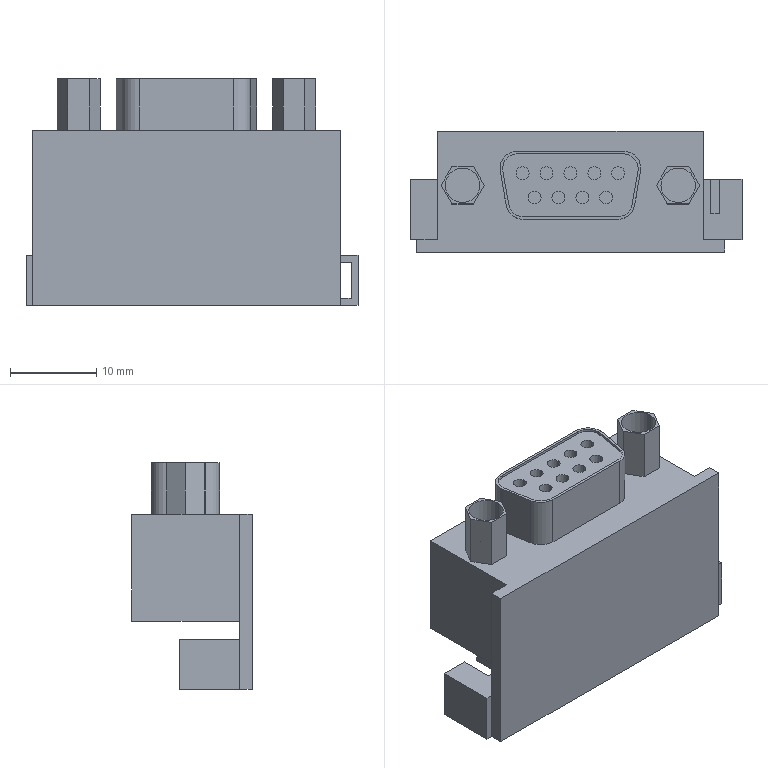Part | SolidWorks | features BaseBody 1 | 1 solid | 111 faces | box 38.5 x 14 x 26.3 mm | volume 7123 mm3 | plane 79 | cylinder 32 | commonest cylinder face diameters 1.5 x18 4 x9 3.4 x5